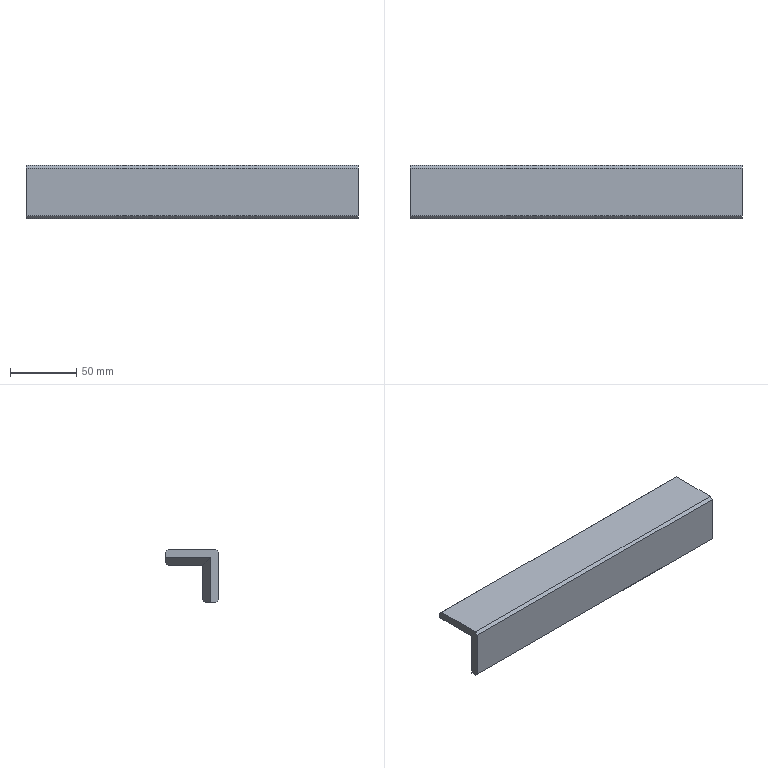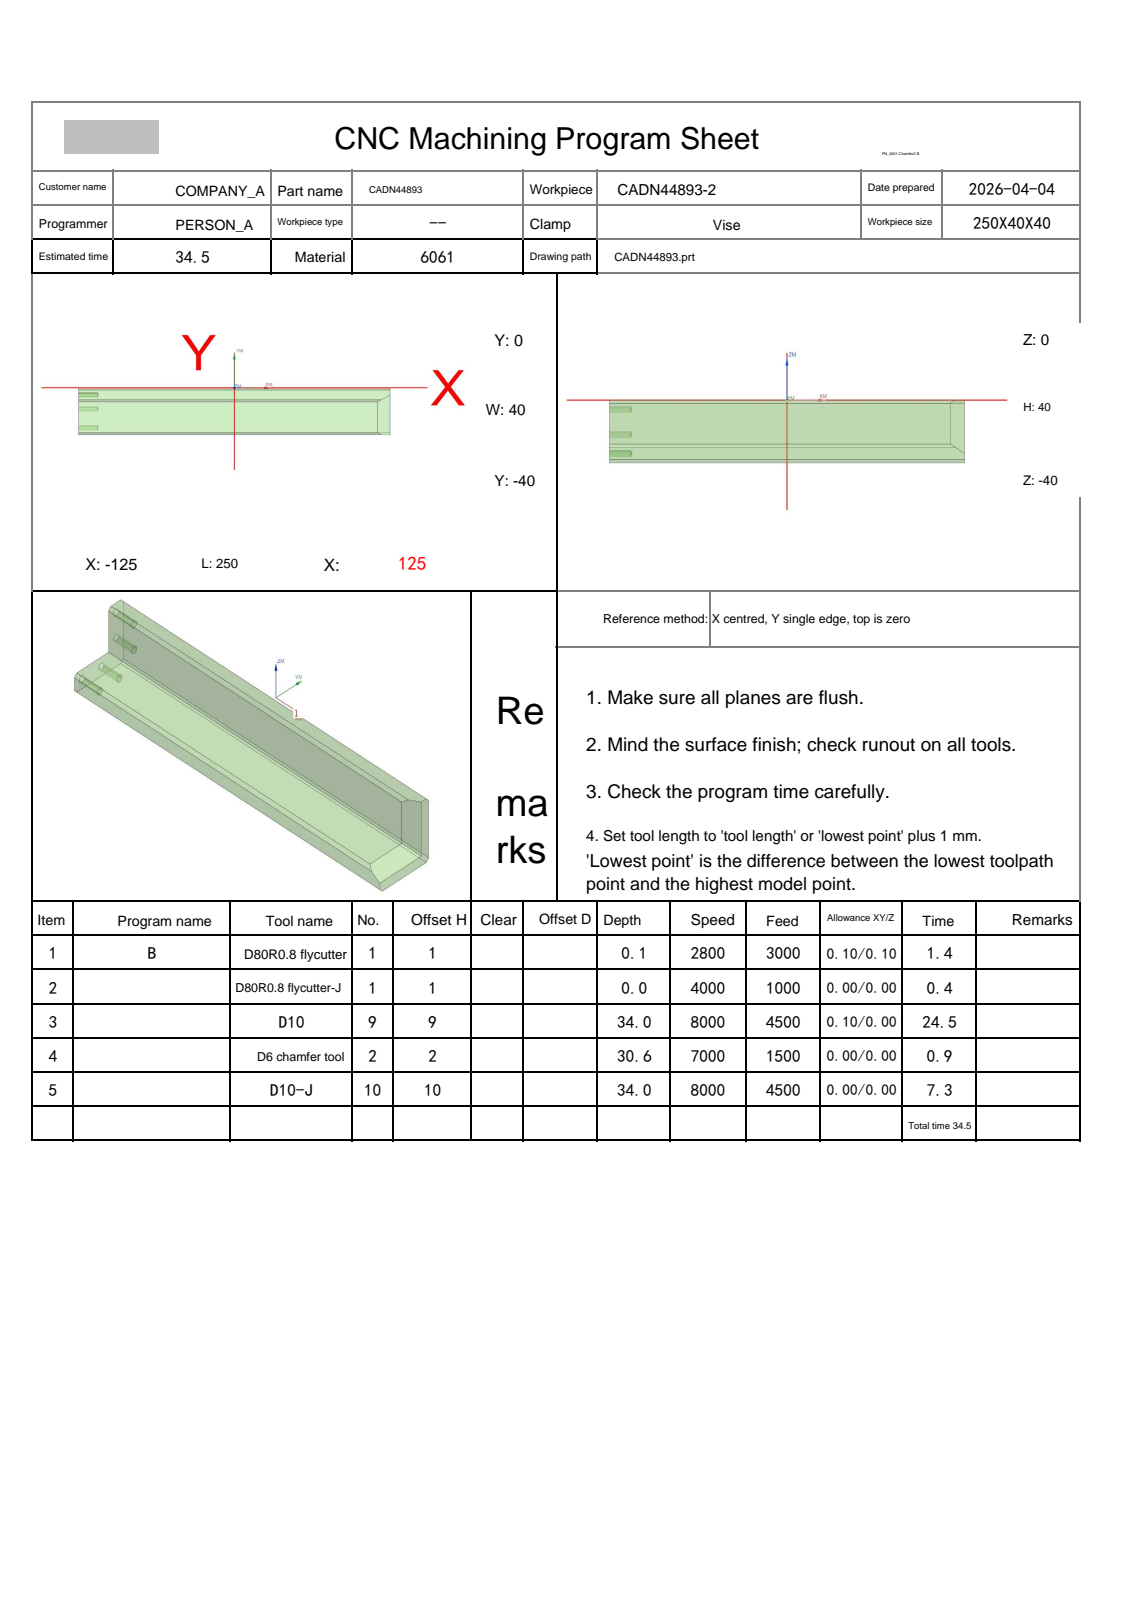NC program | NX | posted by the shop | part box 250 x 40 x 40 mm
Lines 4329 to 4411 of 8932:
N4 T02 M06
(D6 chamfer tool  D=6. R=0. H=02 ce=0.00 di=0.00)
G00 G90 G54 X125.99 Y-1.208 M03 S6500
G43 H02 Z50.
M08
Z.13
G01 Z-1.2 F1500.
G03 X125.915 Y-1.548 I1.907 J-.601
G01 X125.905 Y-1.602
X125.928 Y-1.651
X125.966 Y-1.741
X126. Y-2.
Y-6.
X125.967 Y-6.255
X125.87 Y-6.493
X125.716 Y-6.698
X125.514 Y-6.857
X118.848 Y-10.857
X118.6 Y-10.964
X118.534 Y-10.973
X118.51 Y-10.969
X118.495 Y-10.989
X118.435 Y-11.027
X118.393 Y-11.083
Z.314
G00 Z10.
X-125.99 Y-10.792
Z.13
G01 Z-1.2
G03 X-125.915 Y-10.452 I-1.907 J.601
G01 X-125.905 Y-10.398
X-125.928 Y-10.349
X-125.966 Y-10.259
X-126. Y-10.
Y-2.
X-125.966 Y-1.741
X-125.928 Y-1.651
X-125.905 Y-1.602
X-125.915 Y-1.548
G03 X-125.99 Y-1.208 I-1.983 J-.261
G01 Z.13
G00 Z10.
X-125.916 Y-38.379
Z-25.199
G01 Z-29.199
X-125.966 Y-38.259
X-126. Y-38.
Y-15.123
X-126.008 Y-15.093
X-126.068 Y-15.007
Z-3.084
G00 Z50.
G00 G90 X-128.9 Y1.516 M03 S6500
Z50.
Z-1.2
G01 Z-2.7 F1000.
G03 X-127.763 Y.7 I1.137 J.384
G01 X127.763
G03 X128.9 Y1.516 I0.0 J1.2
G01 Z-1.2
G00 Z50.
X120.284 Y-13.378
Z-1.2
G01 Z-2.7
G03 X119.204 Y-12.7 I-1.08 J-.522
G01 X-127.763
G03 X-128.9 Y-13.516 I0.0 J-1.2
G01 Z-1.2
G00 Z50.
G00 G90 X122.1 Y-40.6 M03 S7000
Z50.
Z-28.1
G01 Z-30.6 F1000.
X115.
X-125.
X-132.1
Z-28.1
G00 Z50.
G91 G28 Z0.0
M05
M09
G91 G28 Z0.0
M01